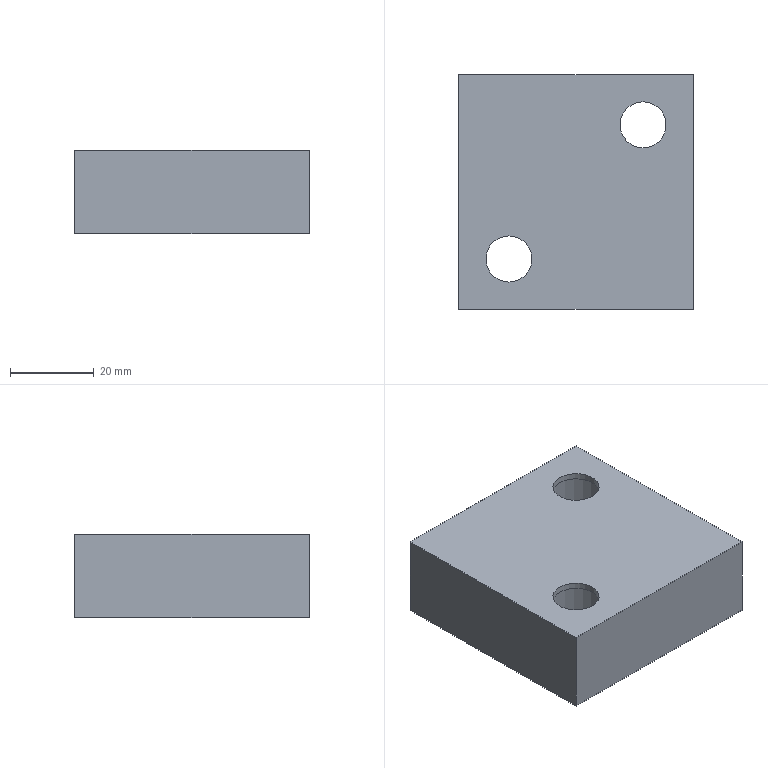Part | NX | features solid 2 | 1 solid | 12 faces | box 56 x 56 x 20 mm | volume 53020 mm3 | plane 8 | cylinder 4 | commonest cylinder face diameters 11 x2 18 x2
STEP:
#1=CARTESIAN_POINT('',(-453.,-328.,-61.));
#2=VERTEX_POINT('',#1);
#3=CARTESIAN_POINT('',(-453.,-328.,-81.));
#4=VERTEX_POINT('',#3);
#5=CARTESIAN_POINT('',(-453.,-328.,-47.5));
#6=DIRECTION('',(0.,0.,-1.));
#7=VECTOR('',#6,1000.);
#8=LINE('',#5,#7);
#9=EDGE_CURVE('',#2,#4,#8,.T.);
#10=ORIENTED_EDGE('',*,*,#9,.T.);
#11=CARTESIAN_POINT('',(-453.,-384.,-81.));
#12=VERTEX_POINT('',#11);
#13=CARTESIAN_POINT('',(-453.,-384.,-81.));
#14=DIRECTION('',(0.,1.,0.));
#15=VECTOR('',#14,1000.);
#16=LINE('',#13,#15);
#17=EDGE_CURVE('',#12,#4,#16,.T.);
#18=ORIENTED_EDGE('',*,*,#17,.F.);
#19=CARTESIAN_POINT('',(-453.,-384.,-61.));
#20=VERTEX_POINT('',#19);
#21=CARTESIAN_POINT('',(-453.,-384.,-47.5));
#22=DIRECTION('',(0.,0.,-1.));
#23=VECTOR('',#22,1000.);
#24=LINE('',#21,#23);
#25=EDGE_CURVE('',#20,#12,#24,.T.);
#26=ORIENTED_EDGE('',*,*,#25,.F.);
#27=CARTESIAN_POINT('',(-453.,-384.,-61.));
#28=DIRECTION('',(0.,1.,0.));
#29=VECTOR('',#28,1000.);
#30=LINE('',#27,#29);
#31=EDGE_CURVE('',#20,#2,#30,.T.);
#32=ORIENTED_EDGE('',*,*,#31,.T.);
#33=EDGE_LOOP('',(#10,#18,#26,#32));
#34=FACE_BOUND('',#33,.T.);
#35=CARTESIAN_POINT('',(-453.,-384.,-47.5));
#36=DIRECTION('',(-1.,0.,0.));
#37=DIRECTION('',(0.,1.,0.));
#38=AXIS2_PLACEMENT_3D('',#35,#36,#37);
#39=PLANE('',#38);
#40=ADVANCED_FACE('',(#34),#39,.T.);
#41=CARTESIAN_POINT('',(-397.,-328.,-61.));
#42=VERTEX_POINT('',#41);
#43=CARTESIAN_POINT('',(-397.,-328.,-81.));
#44=VERTEX_POINT('',#43);
#45=CARTESIAN_POINT('',(-397.,-328.,-47.5));
#46=DIRECTION('',(0.,0.,-1.));
#47=VECTOR('',#46,1000.);
#48=LINE('',#45,#47);
#49=EDGE_CURVE('',#42,#44,#48,.T.);
#50=ORIENTED_EDGE('',*,*,#49,.T.);
#51=CARTESIAN_POINT('',(-453.,-328.,-81.));
#52=DIRECTION('',(1.,0.,0.));
#53=VECTOR('',#52,1000.);
#54=LINE('',#51,#53);
#55=EDGE_CURVE('',#4,#44,#54,.T.);
#56=ORIENTED_EDGE('',*,*,#55,.F.);
#57=ORIENTED_EDGE('',*,*,#9,.F.);
#58=CARTESIAN_POINT('',(-453.,-328.,-61.));
#59=DIRECTION('',(1.,0.,0.));
#60=VECTOR('',#59,1000.);
#61=LINE('',#58,#60);
#62=EDGE_CURVE('',#2,#42,#61,.T.);
#63=ORIENTED_EDGE('',*,*,#62,.T.);
#64=EDGE_LOOP('',(#50,#56,#57,#63));
#65=FACE_BOUND('',#64,.T.);
#66=CARTESIAN_POINT('',(-453.,-328.,-47.5));
#67=DIRECTION('',(0.,1.,0.));
#68=DIRECTION('',(1.,0.,0.));
#69=AXIS2_PLACEMENT_3D('',#66,#67,#68);
#70=PLANE('',#69);
#71=ADVANCED_FACE('',(#65),#70,.T.);
#72=CARTESIAN_POINT('',(-397.,-384.,-61.));
#73=VERTEX_POINT('',#72);
#74=CARTESIAN_POINT('',(-397.,-384.,-81.));
#75=VERTEX_POINT('',#74);
#76=CARTESIAN_POINT('',(-397.,-384.,-47.5));
#77=DIRECTION('',(0.,0.,-1.));
#78=VECTOR('',#77,1000.);
#79=LINE('',#76,#78);
#80=EDGE_CURVE('',#73,#75,#79,.T.);
#81=ORIENTED_EDGE('',*,*,#80,.T.);
#82=CARTESIAN_POINT('',(-397.,-328.,-81.));
#83=DIRECTION('',(0.,-1.,0.));
#84=VECTOR('',#83,1000.);
#85=LINE('',#82,#84);
#86=EDGE_CURVE('',#44,#75,#85,.T.);
#87=ORIENTED_EDGE('',*,*,#86,.F.);
#88=ORIENTED_EDGE('',*,*,#49,.F.);
#89=CARTESIAN_POINT('',(-397.,-328.,-61.));
#90=DIRECTION('',(0.,-1.,0.));
#91=VECTOR('',#90,1000.);
#92=LINE('',#89,#91);
#93=EDGE_CURVE('',#42,#73,#92,.T.);
#94=ORIENTED_EDGE('',*,*,#93,.T.);
#95=EDGE_LOOP('',(#81,#87,#88,#94));
#96=FACE_BOUND('',#95,.T.);
#97=CARTESIAN_POINT('',(-397.,-328.,-47.5));
#98=DIRECTION('',(1.,0.,0.));
#99=DIRECTION('',(0.,-1.,0.));
#100=AXIS2_PLACEMENT_3D('',#97,#98,#99);
#101=PLANE('',#100);
#102=ADVANCED_FACE('',(#96),#101,.T.);
#103=CARTESIAN_POINT('',(-441.,-366.5,-62.5));
#104=VERTEX_POINT('',#103);
#105=CARTESIAN_POINT('',(-441.,-372.,-62.5));
#106=DIRECTION('',(0.,0.,1.));
#107=DIRECTION('',(0.,1.,0.));
#108=AXIS2_PLACEMENT_3D('',#105,#106,#107);
#109=CIRCLE('',#108,5.5);
#110=EDGE_CURVE('',#104,#104,#109,.F.);
#111=ORIENTED_EDGE('',*,*,#110,.T.);
#112=EDGE_LOOP('',(#111));
#113=FACE_BOUND('',#112,.T.);
#114=CARTESIAN_POINT('',(-441.,-377.5,-61.));
#115=VERTEX_POINT('',#114);
#116=CARTESIAN_POINT('',(-441.,-372.,-61.));
#117=DIRECTION('',(0.,0.,1.));
#118=DIRECTION('',(0.,-1.,0.));
#119=AXIS2_PLACEMENT_3D('',#116,#117,#118);
#120=CIRCLE('',#119,5.5);
#121=EDGE_CURVE('',#115,#115,#120,.F.);
#122=ORIENTED_EDGE('',*,*,#121,.F.);
#123=EDGE_LOOP('',(#122));
#124=FACE_BOUND('',#123,.T.);
#125=CARTESIAN_POINT('',(-441.,-372.,-47.5));
#126=DIRECTION('',(0.,0.,-1.));
#127=DIRECTION('',(0.,-1.,0.));
#128=AXIS2_PLACEMENT_3D('',#125,#126,#127);
#129=CYLINDRICAL_SURFACE('',#128,5.5);
#130=ADVANCED_FACE('',(#113,#124),#129,.F.);
#131=CARTESIAN_POINT('',(-409.,-334.5,-62.5));
#132=VERTEX_POINT('',#131);
#133=CARTESIAN_POINT('',(-409.,-340.,-62.5));
#134=DIRECTION('',(0.,0.,1.));
#135=DIRECTION('',(0.,1.,0.));
#136=AXIS2_PLACEMENT_3D('',#133,#134,#135);
#137=CIRCLE('',#136,5.5);
#138=EDGE_CURVE('',#132,#132,#137,.F.);
#139=ORIENTED_EDGE('',*,*,#138,.T.);
#140=EDGE_LOOP('',(#139));
#141=FACE_BOUND('',#140,.T.);
#142=CARTESIAN_POINT('',(-409.,-345.5,-61.));
#143=VERTEX_POINT('',#142);
#144=CARTESIAN_POINT('',(-409.,-340.,-61.));
#145=DIRECTION('',(0.,0.,1.));
#146=DIRECTION('',(0.,-1.,0.));
#147=AXIS2_PLACEMENT_3D('',#144,#145,#146);
#148=CIRCLE('',#147,5.5);
#149=EDGE_CURVE('',#143,#143,#148,.F.);
#150=ORIENTED_EDGE('',*,*,#149,.F.);
#151=EDGE_LOOP('',(#150));
#152=FACE_BOUND('',#151,.T.);
#153=CARTESIAN_POINT('',(-409.,-340.,-47.5));
#154=DIRECTION('',(0.,0.,-1.));
#155=DIRECTION('',(0.,-1.,0.));
#156=AXIS2_PLACEMENT_3D('',#153,#154,#155);
#157=CYLINDRICAL_SURFACE('',#156,5.5);
#158=ADVANCED_FACE('',(#141,#152),#157,.F.);
#159=CARTESIAN_POINT('',(-397.,-384.,-61.));
#160=DIRECTION('',(-1.,0.,0.));
#161=VECTOR('',#160,1000.);
#162=LINE('',#159,#161);
#163=EDGE_CURVE('',#73,#20,#162,.T.);
#164=ORIENTED_EDGE('',*,*,#163,.T.);
#165=ORIENTED_EDGE('',*,*,#25,.T.);
#166=CARTESIAN_POINT('',(-397.,-384.,-81.));
#167=DIRECTION('',(-1.,0.,0.));
#168=VECTOR('',#167,1000.);
#169=LINE('',#166,#168);
#170=EDGE_CURVE('',#75,#12,#169,.T.);
#171=ORIENTED_EDGE('',*,*,#170,.F.);
#172=ORIENTED_EDGE('',*,*,#80,.F.);
#173=EDGE_LOOP('',(#164,#165,#171,#172));
#174=FACE_BOUND('',#173,.T.);
#175=CARTESIAN_POINT('',(-397.,-384.,-47.5));
#176=DIRECTION('',(0.,-1.,0.));
#177=DIRECTION('',(-1.,0.,0.));
#178=AXIS2_PLACEMENT_3D('',#175,#176,#177);
#179=PLANE('',#178);
#180=ADVANCED_FACE('',(#174),#179,.T.);
#181=ORIENTED_EDGE('',*,*,#149,.T.);
#182=EDGE_LOOP('',(#181));
#183=FACE_BOUND('',#182,.T.);
#184=ORIENTED_EDGE('',*,*,#121,.T.);
#185=EDGE_LOOP('',(#184));
#186=FACE_BOUND('',#185,.T.);
#187=ORIENTED_EDGE('',*,*,#31,.F.);
#188=ORIENTED_EDGE('',*,*,#163,.F.);
#189=ORIENTED_EDGE('',*,*,#93,.F.);
#190=ORIENTED_EDGE('',*,*,#62,.F.);
#191=EDGE_LOOP('',(#187,#188,#189,#190));
#192=FACE_BOUND('',#191,.T.);
#193=CARTESIAN_POINT('',(-453.,-384.,-61.));
#194=DIRECTION('',(0.,0.,1.));
#195=DIRECTION('',(0.,1.,0.));
#196=AXIS2_PLACEMENT_3D('',#193,#194,#195);
#197=PLANE('',#196);
#198=ADVANCED_FACE('',(#183,#186,#192),#197,.T.);
#199=CARTESIAN_POINT('',(-409.,-331.,-81.));
#200=VERTEX_POINT('',#199);
#201=CARTESIAN_POINT('',(-409.,-340.,-81.));
#202=DIRECTION('',(0.,0.,1.));
#203=DIRECTION('',(0.,1.,0.));
#204=AXIS2_PLACEMENT_3D('',#201,#202,#203);
#205=CIRCLE('',#204,9.);
#206=EDGE_CURVE('',#200,#200,#205,.T.);
#207=ORIENTED_EDGE('',*,*,#206,.T.);
#208=EDGE_LOOP('',(#207));
#209=FACE_BOUND('',#208,.T.);
#210=CARTESIAN_POINT('',(-441.,-363.,-81.));
#211=VERTEX_POINT('',#210);
#212=CARTESIAN_POINT('',(-441.,-372.,-81.));
#213=DIRECTION('',(0.,0.,1.));
#214=DIRECTION('',(0.,1.,0.));
#215=AXIS2_PLACEMENT_3D('',#212,#213,#214);
#216=CIRCLE('',#215,9.);
#217=EDGE_CURVE('',#211,#211,#216,.T.);
#218=ORIENTED_EDGE('',*,*,#217,.T.);
#219=EDGE_LOOP('',(#218));
#220=FACE_BOUND('',#219,.T.);
#221=ORIENTED_EDGE('',*,*,#17,.T.);
#222=ORIENTED_EDGE('',*,*,#55,.T.);
#223=ORIENTED_EDGE('',*,*,#86,.T.);
#224=ORIENTED_EDGE('',*,*,#170,.T.);
#225=EDGE_LOOP('',(#221,#222,#223,#224));
#226=FACE_BOUND('',#225,.T.);
#227=CARTESIAN_POINT('',(-453.,-384.,-81.));
#228=DIRECTION('',(0.,0.,1.));
#229=DIRECTION('',(0.,1.,0.));
#230=AXIS2_PLACEMENT_3D('',#227,#228,#229);
#231=PLANE('',#230);
#232=ADVANCED_FACE('',(#209,#220,#226),#231,.F.);
#233=CARTESIAN_POINT('',(-441.,-363.,-62.5));
#234=VERTEX_POINT('',#233);
#235=CARTESIAN_POINT('',(-441.,-372.,-62.5));
#236=DIRECTION('',(0.,0.,1.));
#237=DIRECTION('',(0.,1.,0.));
#238=AXIS2_PLACEMENT_3D('',#235,#236,#237);
#239=CIRCLE('',#238,9.);
#240=EDGE_CURVE('',#234,#234,#239,.T.);
#241=ORIENTED_EDGE('',*,*,#240,.F.);
#242=EDGE_LOOP('',(#241));
#243=FACE_BOUND('',#242,.T.);
#244=ORIENTED_EDGE('',*,*,#110,.F.);
#245=EDGE_LOOP('',(#244));
#246=FACE_BOUND('',#245,.T.);
#247=CARTESIAN_POINT('',(-409.,-340.,-62.5));
#248=DIRECTION('',(0.,0.,1.));
#249=DIRECTION('',(0.,1.,0.));
#250=AXIS2_PLACEMENT_3D('',#247,#248,#249);
#251=PLANE('',#250);
#252=ADVANCED_FACE('',(#243,#246),#251,.F.);
#253=ORIENTED_EDGE('',*,*,#240,.T.);
#254=EDGE_LOOP('',(#253));
#255=FACE_BOUND('',#254,.T.);
#256=ORIENTED_EDGE('',*,*,#217,.F.);
#257=EDGE_LOOP('',(#256));
#258=FACE_BOUND('',#257,.T.);
#259=CARTESIAN_POINT('',(-441.,-372.,-67.5));
#260=DIRECTION('',(0.,0.,1.));
#261=DIRECTION('',(0.,1.,0.));
#262=AXIS2_PLACEMENT_3D('',#259,#260,#261);
#263=CYLINDRICAL_SURFACE('',#262,9.);
#264=ADVANCED_FACE('',(#255,#258),#263,.F.);
#265=CARTESIAN_POINT('',(-409.,-331.,-62.5));
#266=VERTEX_POINT('',#265);
#267=CARTESIAN_POINT('',(-409.,-340.,-62.5));
#268=DIRECTION('',(0.,0.,1.));
#269=DIRECTION('',(0.,1.,0.));
#270=AXIS2_PLACEMENT_3D('',#267,#268,#269);
#271=CIRCLE('',#270,9.);
#272=EDGE_CURVE('',#266,#266,#271,.T.);
#273=ORIENTED_EDGE('',*,*,#272,.F.);
#274=EDGE_LOOP('',(#273));
#275=FACE_BOUND('',#274,.T.);
#276=ORIENTED_EDGE('',*,*,#138,.F.);
#277=EDGE_LOOP('',(#276));
#278=FACE_BOUND('',#277,.T.);
#279=CARTESIAN_POINT('',(-409.,-340.,-62.5));
#280=DIRECTION('',(0.,0.,1.));
#281=DIRECTION('',(0.,1.,0.));
#282=AXIS2_PLACEMENT_3D('',#279,#280,#281);
#283=PLANE('',#282);
#284=ADVANCED_FACE('',(#275,#278),#283,.F.);
#285=ORIENTED_EDGE('',*,*,#272,.T.);
#286=EDGE_LOOP('',(#285));
#287=FACE_BOUND('',#286,.T.);
#288=ORIENTED_EDGE('',*,*,#206,.F.);
#289=EDGE_LOOP('',(#288));
#290=FACE_BOUND('',#289,.T.);
#291=CARTESIAN_POINT('',(-409.,-340.,-67.5));
#292=DIRECTION('',(0.,0.,1.));
#293=DIRECTION('',(0.,1.,0.));
#294=AXIS2_PLACEMENT_3D('',#291,#292,#293);
#295=CYLINDRICAL_SURFACE('',#294,9.);
#296=ADVANCED_FACE('',(#287,#290),#295,.F.);
#297=CLOSED_SHELL('',(#40,#71,#102,#130,#158,#180,#198,#232,#252,#264,#284,#296));
#298=MANIFOLD_SOLID_BREP('',#297);
#299=(LENGTH_UNIT()NAMED_UNIT(*)SI_UNIT(.MILLI.,.METRE.));
#300=UNCERTAINTY_MEASURE_WITH_UNIT(LENGTH_MEASURE(0.00001),#299,'','');
#301=(NAMED_UNIT(*)PLANE_ANGLE_UNIT()SI_UNIT($,.RADIAN.));
#302=(NAMED_UNIT(*)SI_UNIT($,.STERADIAN.)SOLID_ANGLE_UNIT());
#303=(GEOMETRIC_REPRESENTATION_CONTEXT(3)GLOBAL_UNCERTAINTY_ASSIGNED_CONTEXT((#300))GLOBAL_UNIT_ASSIGNED_CONTEXT((#299,#301,#302))REPRESENTATION_CONTEXT('',''));
#304=ADVANCED_BREP_SHAPE_REPRESENTATION('',(#298),#303);